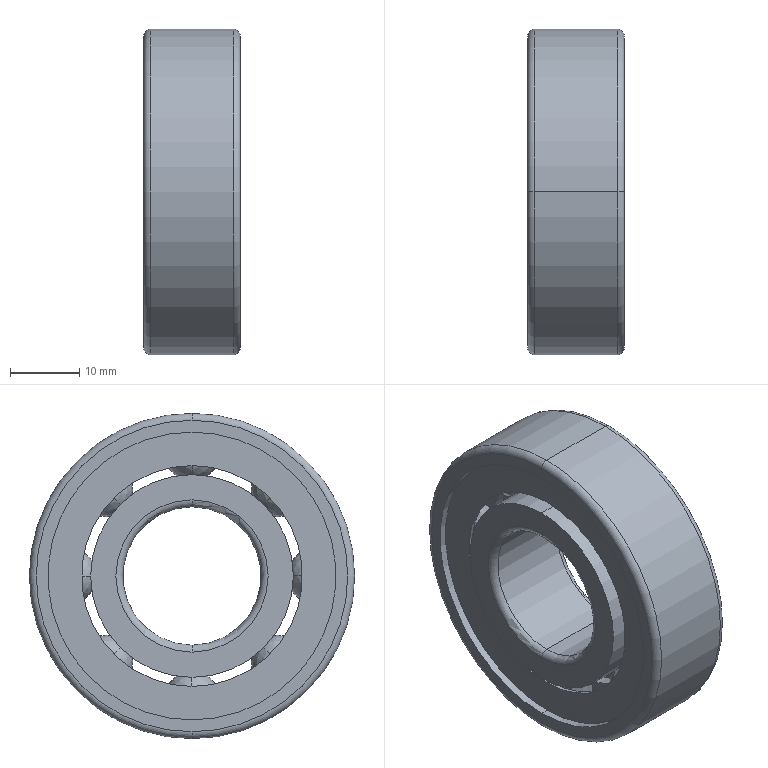Part | SolidWorks | features BaseBody 3 | 3 solids | 158 faces | box 14 x 47 x 47 mm | volume 12570 mm3 | sphere 96 | cylinder 24 | plane 24 | torus 14 | commonest cylinder face diameters 41.6 x8 29.3 x4 31.92 x4 20 x2 33.267 x2 37.633 x2